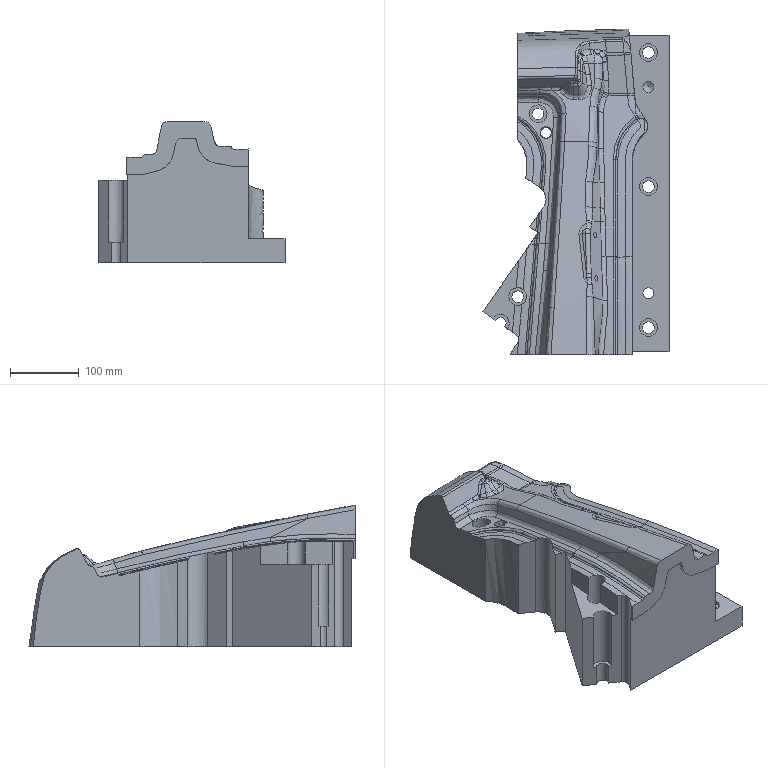Part | NX | features solid 2 | 1 solid | 271 faces | box 270.499 x 474.982 x 209.998 mm | volume 9574242 mm3 | spline 222 | plane 29 | cylinder 19 | cone 1 | commonest cylinder face diameters 17 x6 26 x6 16 x3 32 x2 20 x1 40 x1